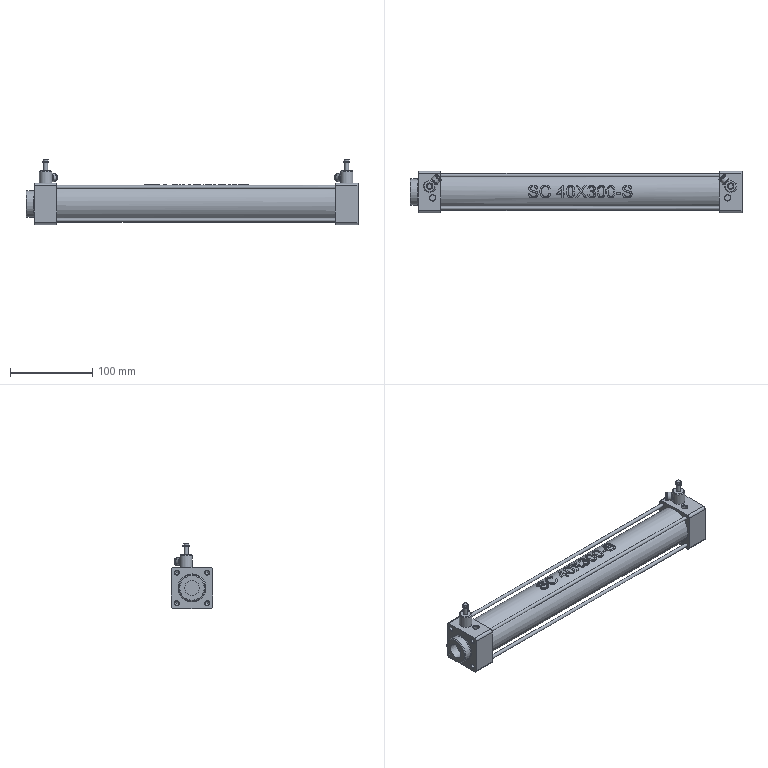Part | STEP file | Tube feed_id346_x_t | 1 solid | 236 faces | box 403 x 50 x 79 mm | volume 690158 mm3 | plane 94 | cylinder 75 | spline 35 | cone 24 | torus 8 | commonest cylinder face diameters 6 x12 10 x12 5 x10 47 x10 8 x8 20 x8